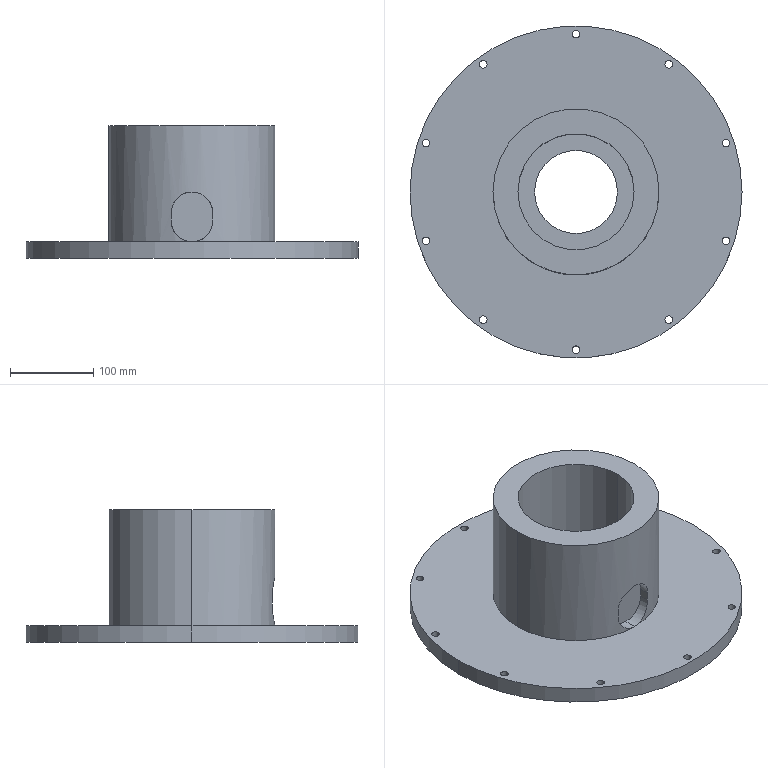Part | SolidWorks | features ICE 2, Cut 1, Extrusion 1, Fillet 1 | 1 solid | 39 faces | box 400 x 400 x 160 mm | volume 4551688 mm3 | cylinder 32 | plane 7 | commonest cylinder face diameters 9 x20 50 x4 100 x2 140 x2 200 x2 400 x2
STEP:
#1=CARTESIAN_POINT('',(-50.,0.,0.));
#2=VERTEX_POINT('',#1);
#3=CARTESIAN_POINT('',(50.,0.,0.));
#4=VERTEX_POINT('',#3);
#5=CARTESIAN_POINT('',(0.,0.,0.));
#6=DIRECTION('',(0.,0.,1.));
#7=DIRECTION('',(1.,0.,0.));
#8=AXIS2_PLACEMENT_3D('',#5,#6,#7);
#9=CIRCLE('',#8,50.);
#10=EDGE_CURVE('',#2,#4,#9,.T.);
#11=ORIENTED_EDGE('',*,*,#10,.F.);
#12=CARTESIAN_POINT('',(-50.,0.,20.));
#13=VERTEX_POINT('',#12);
#14=CARTESIAN_POINT('',(-50.,0.,0.));
#15=DIRECTION('',(0.,0.,1.));
#16=VECTOR('',#15,1000.);
#17=LINE('',#14,#16);
#18=EDGE_CURVE('',#2,#13,#17,.T.);
#19=ORIENTED_EDGE('',*,*,#18,.T.);
#20=CARTESIAN_POINT('',(50.,0.,20.));
#21=VERTEX_POINT('',#20);
#22=CARTESIAN_POINT('',(0.,0.,20.));
#23=DIRECTION('',(0.,0.,1.));
#24=DIRECTION('',(1.,0.,0.));
#25=AXIS2_PLACEMENT_3D('',#22,#23,#24);
#26=CIRCLE('',#25,50.);
#27=EDGE_CURVE('',#13,#21,#26,.T.);
#28=ORIENTED_EDGE('',*,*,#27,.T.);
#29=CARTESIAN_POINT('',(50.,0.,0.));
#30=DIRECTION('',(0.,0.,1.));
#31=VECTOR('',#30,1000.);
#32=LINE('',#29,#31);
#33=EDGE_CURVE('',#4,#21,#32,.T.);
#34=ORIENTED_EDGE('',*,*,#33,.F.);
#35=EDGE_LOOP('',(#11,#19,#28,#34));
#36=FACE_OUTER_BOUND('',#35,.T.);
#37=CARTESIAN_POINT('',(0.,0.,0.));
#38=DIRECTION('',(0.,0.,1.));
#39=DIRECTION('',(1.,0.,0.));
#40=AXIS2_PLACEMENT_3D('',#37,#38,#39);
#41=CYLINDRICAL_SURFACE('',#40,50.);
#42=ADVANCED_FACE('',(#36),#41,.F.);
#43=CARTESIAN_POINT('',(-70.,0.,160.));
#44=VERTEX_POINT('',#43);
#45=CARTESIAN_POINT('',(70.,0.,160.));
#46=VERTEX_POINT('',#45);
#47=CARTESIAN_POINT('',(0.,0.,160.));
#48=DIRECTION('',(0.,0.,1.));
#49=DIRECTION('',(1.,0.,0.));
#50=AXIS2_PLACEMENT_3D('',#47,#48,#49);
#51=CIRCLE('',#50,70.);
#52=EDGE_CURVE('',#44,#46,#51,.T.);
#53=ORIENTED_EDGE('',*,*,#52,.T.);
#54=CARTESIAN_POINT('',(70.,0.,20.));
#55=VERTEX_POINT('',#54);
#56=CARTESIAN_POINT('',(70.,0.,160.));
#57=DIRECTION('',(0.,0.,-1.));
#58=VECTOR('',#57,1000.);
#59=LINE('',#56,#58);
#60=EDGE_CURVE('',#46,#55,#59,.T.);
#61=ORIENTED_EDGE('',*,*,#60,.T.);
#62=CARTESIAN_POINT('',(-70.,0.,20.));
#63=VERTEX_POINT('',#62);
#64=CARTESIAN_POINT('',(0.,0.,20.));
#65=DIRECTION('',(0.,0.,-1.));
#66=DIRECTION('',(1.,0.,0.));
#67=AXIS2_PLACEMENT_3D('',#64,#65,#66);
#68=CIRCLE('',#67,70.);
#69=EDGE_CURVE('',#55,#63,#68,.T.);
#70=ORIENTED_EDGE('',*,*,#69,.T.);
#71=CARTESIAN_POINT('',(-70.,0.,160.));
#72=DIRECTION('',(0.,0.,-1.));
#73=VECTOR('',#72,1000.);
#74=LINE('',#71,#73);
#75=EDGE_CURVE('',#44,#63,#74,.T.);
#76=ORIENTED_EDGE('',*,*,#75,.F.);
#77=EDGE_LOOP('',(#53,#61,#70,#76));
#78=FACE_OUTER_BOUND('',#77,.T.);
#79=CARTESIAN_POINT('',(0.,0.,160.));
#80=DIRECTION('',(0.,0.,-1.));
#81=DIRECTION('',(-1.,0.,0.));
#82=AXIS2_PLACEMENT_3D('',#79,#80,#81);
#83=CYLINDRICAL_SURFACE('',#82,70.);
#84=ADVANCED_FACE('',(#78),#83,.F.);
#85=CARTESIAN_POINT('',(100.,0.,160.));
#86=VERTEX_POINT('',#85);
#87=CARTESIAN_POINT('',(-100.,0.,160.));
#88=VERTEX_POINT('',#87);
#89=CARTESIAN_POINT('',(0.,0.,160.));
#90=DIRECTION('',(0.,0.,1.));
#91=DIRECTION('',(1.,0.,0.));
#92=AXIS2_PLACEMENT_3D('',#89,#90,#91);
#93=CIRCLE('',#92,100.);
#94=EDGE_CURVE('',#86,#88,#93,.T.);
#95=ORIENTED_EDGE('',*,*,#94,.F.);
#96=CARTESIAN_POINT('',(100.,0.,20.));
#97=VERTEX_POINT('',#96);
#98=CARTESIAN_POINT('',(100.,0.,160.));
#99=DIRECTION('',(0.,0.,-1.));
#100=VECTOR('',#99,1000.);
#101=LINE('',#98,#100);
#102=EDGE_CURVE('',#86,#97,#101,.T.);
#103=ORIENTED_EDGE('',*,*,#102,.T.);
#104=CARTESIAN_POINT('',(-100.,0.,20.));
#105=VERTEX_POINT('',#104);
#106=CARTESIAN_POINT('',(0.,0.,20.));
#107=DIRECTION('',(0.,0.,1.));
#108=DIRECTION('',(1.,0.,0.));
#109=AXIS2_PLACEMENT_3D('',#106,#107,#108);
#110=CIRCLE('',#109,100.);
#111=EDGE_CURVE('',#97,#105,#110,.T.);
#112=ORIENTED_EDGE('',*,*,#111,.T.);
#113=CARTESIAN_POINT('',(-100.,0.,160.));
#114=DIRECTION('',(0.,0.,-1.));
#115=VECTOR('',#114,1000.);
#116=LINE('',#113,#115);
#117=EDGE_CURVE('',#88,#105,#116,.T.);
#118=ORIENTED_EDGE('',*,*,#117,.F.);
#119=EDGE_LOOP('',(#95,#103,#112,#118));
#120=FACE_OUTER_BOUND('',#119,.T.);
#121=CARTESIAN_POINT('',(0.,0.,160.));
#122=DIRECTION('',(0.,0.,-1.));
#123=DIRECTION('',(-1.,0.,0.));
#124=AXIS2_PLACEMENT_3D('',#121,#122,#123);
#125=CYLINDRICAL_SURFACE('',#124,100.);
#126=ADVANCED_FACE('',(#120),#125,.T.);
#127=CARTESIAN_POINT('',(-116.179,153.713,20.));
#128=VERTEX_POINT('',#127);
#129=CARTESIAN_POINT('',(-107.179,153.713,20.));
#130=VERTEX_POINT('',#129);
#131=CARTESIAN_POINT('',(-111.679,153.713,20.));
#132=DIRECTION('',(0.,0.,1.));
#133=DIRECTION('',(1.,0.,0.));
#134=AXIS2_PLACEMENT_3D('',#131,#132,#133);
#135=CIRCLE('',#134,4.5);
#136=EDGE_CURVE('',#128,#130,#135,.T.);
#137=ORIENTED_EDGE('',*,*,#136,.T.);
#138=CARTESIAN_POINT('',(-107.179,153.713,0.));
#139=VERTEX_POINT('',#138);
#140=CARTESIAN_POINT('',(-107.179,153.713,20.));
#141=DIRECTION('',(0.,0.,-1.));
#142=VECTOR('',#141,1000.);
#143=LINE('',#140,#142);
#144=EDGE_CURVE('',#130,#139,#143,.T.);
#145=ORIENTED_EDGE('',*,*,#144,.T.);
#146=CARTESIAN_POINT('',(-116.179,153.713,0.));
#147=VERTEX_POINT('',#146);
#148=CARTESIAN_POINT('',(-111.679,153.713,0.));
#149=DIRECTION('',(0.,0.,1.));
#150=DIRECTION('',(1.,0.,0.));
#151=AXIS2_PLACEMENT_3D('',#148,#149,#150);
#152=CIRCLE('',#151,4.5);
#153=EDGE_CURVE('',#147,#139,#152,.T.);
#154=ORIENTED_EDGE('',*,*,#153,.F.);
#155=CARTESIAN_POINT('',(-116.179,153.713,20.));
#156=DIRECTION('',(0.,0.,-1.));
#157=VECTOR('',#156,1000.);
#158=LINE('',#155,#157);
#159=EDGE_CURVE('',#128,#147,#158,.T.);
#160=ORIENTED_EDGE('',*,*,#159,.F.);
#161=EDGE_LOOP('',(#137,#145,#154,#160));
#162=FACE_OUTER_BOUND('',#161,.T.);
#163=CARTESIAN_POINT('',(-111.679,153.713,20.));
#164=DIRECTION('',(0.,0.,-1.));
#165=DIRECTION('',(-1.,0.,0.));
#166=AXIS2_PLACEMENT_3D('',#163,#164,#165);
#167=CYLINDRICAL_SURFACE('',#166,4.5);
#168=ADVANCED_FACE('',(#162),#167,.F.);
#169=CARTESIAN_POINT('',(-185.201,58.713,20.));
#170=VERTEX_POINT('',#169);
#171=CARTESIAN_POINT('',(-176.201,58.713,20.));
#172=VERTEX_POINT('',#171);
#173=CARTESIAN_POINT('',(-180.701,58.713,20.));
#174=DIRECTION('',(0.,0.,1.));
#175=DIRECTION('',(1.,0.,0.));
#176=AXIS2_PLACEMENT_3D('',#173,#174,#175);
#177=CIRCLE('',#176,4.5);
#178=EDGE_CURVE('',#170,#172,#177,.T.);
#179=ORIENTED_EDGE('',*,*,#178,.T.);
#180=CARTESIAN_POINT('',(-176.201,58.713,0.));
#181=VERTEX_POINT('',#180);
#182=CARTESIAN_POINT('',(-176.201,58.713,20.));
#183=DIRECTION('',(0.,0.,-1.));
#184=VECTOR('',#183,1000.);
#185=LINE('',#182,#184);
#186=EDGE_CURVE('',#172,#181,#185,.T.);
#187=ORIENTED_EDGE('',*,*,#186,.T.);
#188=CARTESIAN_POINT('',(-185.201,58.713,0.));
#189=VERTEX_POINT('',#188);
#190=CARTESIAN_POINT('',(-180.701,58.713,0.));
#191=DIRECTION('',(0.,0.,1.));
#192=DIRECTION('',(1.,0.,0.));
#193=AXIS2_PLACEMENT_3D('',#190,#191,#192);
#194=CIRCLE('',#193,4.5);
#195=EDGE_CURVE('',#189,#181,#194,.T.);
#196=ORIENTED_EDGE('',*,*,#195,.F.);
#197=CARTESIAN_POINT('',(-185.201,58.713,20.));
#198=DIRECTION('',(0.,0.,-1.));
#199=VECTOR('',#198,1000.);
#200=LINE('',#197,#199);
#201=EDGE_CURVE('',#170,#189,#200,.T.);
#202=ORIENTED_EDGE('',*,*,#201,.F.);
#203=EDGE_LOOP('',(#179,#187,#196,#202));
#204=FACE_OUTER_BOUND('',#203,.T.);
#205=CARTESIAN_POINT('',(-180.701,58.713,20.));
#206=DIRECTION('',(0.,0.,-1.));
#207=DIRECTION('',(-1.,0.,0.));
#208=AXIS2_PLACEMENT_3D('',#205,#206,#207);
#209=CYLINDRICAL_SURFACE('',#208,4.5);
#210=ADVANCED_FACE('',(#204),#209,.F.);
#211=CARTESIAN_POINT('',(-185.201,-58.713,20.));
#212=VERTEX_POINT('',#211);
#213=CARTESIAN_POINT('',(-176.201,-58.713,20.));
#214=VERTEX_POINT('',#213);
#215=CARTESIAN_POINT('',(-180.701,-58.713,20.));
#216=DIRECTION('',(0.,0.,1.));
#217=DIRECTION('',(1.,0.,0.));
#218=AXIS2_PLACEMENT_3D('',#215,#216,#217);
#219=CIRCLE('',#218,4.5);
#220=EDGE_CURVE('',#212,#214,#219,.T.);
#221=ORIENTED_EDGE('',*,*,#220,.T.);
#222=CARTESIAN_POINT('',(-176.201,-58.713,0.));
#223=VERTEX_POINT('',#222);
#224=CARTESIAN_POINT('',(-176.201,-58.713,20.));
#225=DIRECTION('',(0.,0.,-1.));
#226=VECTOR('',#225,1000.);
#227=LINE('',#224,#226);
#228=EDGE_CURVE('',#214,#223,#227,.T.);
#229=ORIENTED_EDGE('',*,*,#228,.T.);
#230=CARTESIAN_POINT('',(-185.201,-58.713,0.));
#231=VERTEX_POINT('',#230);
#232=CARTESIAN_POINT('',(-180.701,-58.713,0.));
#233=DIRECTION('',(0.,0.,1.));
#234=DIRECTION('',(1.,0.,0.));
#235=AXIS2_PLACEMENT_3D('',#232,#233,#234);
#236=CIRCLE('',#235,4.5);
#237=EDGE_CURVE('',#231,#223,#236,.T.);
#238=ORIENTED_EDGE('',*,*,#237,.F.);
#239=CARTESIAN_POINT('',(-185.201,-58.713,20.));
#240=DIRECTION('',(0.,0.,-1.));
#241=VECTOR('',#240,1000.);
#242=LINE('',#239,#241);
#243=EDGE_CURVE('',#212,#231,#242,.T.);
#244=ORIENTED_EDGE('',*,*,#243,.F.);
#245=EDGE_LOOP('',(#221,#229,#238,#244));
#246=FACE_OUTER_BOUND('',#245,.T.);
#247=CARTESIAN_POINT('',(-180.701,-58.713,20.));
#248=DIRECTION('',(0.,0.,-1.));
#249=DIRECTION('',(-1.,0.,0.));
#250=AXIS2_PLACEMENT_3D('',#247,#248,#249);
#251=CYLINDRICAL_SURFACE('',#250,4.5);
#252=ADVANCED_FACE('',(#246),#251,.F.);
#253=CARTESIAN_POINT('',(-116.179,-153.713,20.));
#254=VERTEX_POINT('',#253);
#255=CARTESIAN_POINT('',(-107.179,-153.713,20.));
#256=VERTEX_POINT('',#255);
#257=CARTESIAN_POINT('',(-111.679,-153.713,20.));
#258=DIRECTION('',(0.,0.,1.));
#259=DIRECTION('',(1.,0.,0.));
#260=AXIS2_PLACEMENT_3D('',#257,#258,#259);
#261=CIRCLE('',#260,4.5);
#262=EDGE_CURVE('',#254,#256,#261,.T.);
#263=ORIENTED_EDGE('',*,*,#262,.T.);
#264=CARTESIAN_POINT('',(-107.179,-153.713,0.));
#265=VERTEX_POINT('',#264);
#266=CARTESIAN_POINT('',(-107.179,-153.713,20.));
#267=DIRECTION('',(0.,0.,-1.));
#268=VECTOR('',#267,1000.);
#269=LINE('',#266,#268);
#270=EDGE_CURVE('',#256,#265,#269,.T.);
#271=ORIENTED_EDGE('',*,*,#270,.T.);
#272=CARTESIAN_POINT('',(-116.179,-153.713,0.));
#273=VERTEX_POINT('',#272);
#274=CARTESIAN_POINT('',(-111.679,-153.713,0.));
#275=DIRECTION('',(0.,0.,1.));
#276=DIRECTION('',(1.,0.,0.));
#277=AXIS2_PLACEMENT_3D('',#274,#275,#276);
#278=CIRCLE('',#277,4.5);
#279=EDGE_CURVE('',#273,#265,#278,.T.);
#280=ORIENTED_EDGE('',*,*,#279,.F.);
#281=CARTESIAN_POINT('',(-116.179,-153.713,20.));
#282=DIRECTION('',(0.,0.,-1.));
#283=VECTOR('',#282,1000.);
#284=LINE('',#281,#283);
#285=EDGE_CURVE('',#254,#273,#284,.T.);
#286=ORIENTED_EDGE('',*,*,#285,.F.);
#287=EDGE_LOOP('',(#263,#271,#280,#286));
#288=FACE_OUTER_BOUND('',#287,.T.);
#289=CARTESIAN_POINT('',(-111.679,-153.713,20.));
#290=DIRECTION('',(0.,0.,-1.));
#291=DIRECTION('',(-1.,0.,0.));
#292=AXIS2_PLACEMENT_3D('',#289,#290,#291);
#293=CYLINDRICAL_SURFACE('',#292,4.5);
#294=ADVANCED_FACE('',(#288),#293,.F.);
#295=CARTESIAN_POINT('',(-4.5,-190.,20.));
#296=VERTEX_POINT('',#295);
#297=CARTESIAN_POINT('',(4.5,-190.,20.));
#298=VERTEX_POINT('',#297);
#299=CARTESIAN_POINT('',(0.,-190.,20.));
#300=DIRECTION('',(0.,0.,1.));
#301=DIRECTION('',(1.,0.,0.));
#302=AXIS2_PLACEMENT_3D('',#299,#300,#301);
#303=CIRCLE('',#302,4.5);
#304=EDGE_CURVE('',#296,#298,#303,.T.);
#305=ORIENTED_EDGE('',*,*,#304,.T.);
#306=CARTESIAN_POINT('',(4.5,-190.,0.));
#307=VERTEX_POINT('',#306);
#308=CARTESIAN_POINT('',(4.5,-190.,20.));
#309=DIRECTION('',(0.,0.,-1.));
#310=VECTOR('',#309,1000.);
#311=LINE('',#308,#310);
#312=EDGE_CURVE('',#298,#307,#311,.T.);
#313=ORIENTED_EDGE('',*,*,#312,.T.);
#314=CARTESIAN_POINT('',(-4.5,-190.,0.));
#315=VERTEX_POINT('',#314);
#316=CARTESIAN_POINT('',(0.,-190.,0.));
#317=DIRECTION('',(0.,0.,1.));
#318=DIRECTION('',(1.,0.,0.));
#319=AXIS2_PLACEMENT_3D('',#316,#317,#318);
#320=CIRCLE('',#319,4.5);
#321=EDGE_CURVE('',#315,#307,#320,.T.);
#322=ORIENTED_EDGE('',*,*,#321,.F.);
#323=CARTESIAN_POINT('',(-4.5,-190.,20.));
#324=DIRECTION('',(0.,0.,-1.));
#325=VECTOR('',#324,1000.);
#326=LINE('',#323,#325);
#327=EDGE_CURVE('',#296,#315,#326,.T.);
#328=ORIENTED_EDGE('',*,*,#327,.F.);
#329=EDGE_LOOP('',(#305,#313,#322,#328));
#330=FACE_OUTER_BOUND('',#329,.T.);
#331=CARTESIAN_POINT('',(0.,-190.,20.));
#332=DIRECTION('',(0.,0.,-1.));
#333=DIRECTION('',(-1.,0.,0.));
#334=AXIS2_PLACEMENT_3D('',#331,#332,#333);
#335=CYLINDRICAL_SURFACE('',#334,4.5);
#336=ADVANCED_FACE('',(#330),#335,.F.);
#337=CARTESIAN_POINT('',(107.179,-153.713,20.));
#338=VERTEX_POINT('',#337);
#339=CARTESIAN_POINT('',(116.179,-153.713,20.));
#340=VERTEX_POINT('',#339);
#341=CARTESIAN_POINT('',(111.679,-153.713,20.));
#342=DIRECTION('',(0.,0.,1.));
#343=DIRECTION('',(1.,0.,0.));
#344=AXIS2_PLACEMENT_3D('',#341,#342,#343);
#345=CIRCLE('',#344,4.5);
#346=EDGE_CURVE('',#338,#340,#345,.T.);
#347=ORIENTED_EDGE('',*,*,#346,.T.);
#348=CARTESIAN_POINT('',(116.179,-153.713,0.));
#349=VERTEX_POINT('',#348);
#350=CARTESIAN_POINT('',(116.179,-153.713,20.));
#351=DIRECTION('',(0.,0.,-1.));
#352=VECTOR('',#351,1000.);
#353=LINE('',#350,#352);
#354=EDGE_CURVE('',#340,#349,#353,.T.);
#355=ORIENTED_EDGE('',*,*,#354,.T.);
#356=CARTESIAN_POINT('',(107.179,-153.713,0.));
#357=VERTEX_POINT('',#356);
#358=CARTESIAN_POINT('',(111.679,-153.713,0.));
#359=DIRECTION('',(0.,0.,1.));
#360=DIRECTION('',(1.,0.,0.));
#361=AXIS2_PLACEMENT_3D('',#358,#359,#360);
#362=CIRCLE('',#361,4.5);
#363=EDGE_CURVE('',#357,#349,#362,.T.);
#364=ORIENTED_EDGE('',*,*,#363,.F.);
#365=CARTESIAN_POINT('',(107.179,-153.713,20.));
#366=DIRECTION('',(0.,0.,-1.));
#367=VECTOR('',#366,1000.);
#368=LINE('',#365,#367);
#369=EDGE_CURVE('',#338,#357,#368,.T.);
#370=ORIENTED_EDGE('',*,*,#369,.F.);
#371=EDGE_LOOP('',(#347,#355,#364,#370));
#372=FACE_OUTER_BOUND('',#371,.T.);
#373=CARTESIAN_POINT('',(111.679,-153.713,20.));
#374=DIRECTION('',(0.,0.,-1.));
#375=DIRECTION('',(-1.,0.,0.));
#376=AXIS2_PLACEMENT_3D('',#373,#374,#375);
#377=CYLINDRICAL_SURFACE('',#376,4.5);
#378=ADVANCED_FACE('',(#372),#377,.F.);
#379=CARTESIAN_POINT('',(176.201,-58.713,20.));
#380=VERTEX_POINT('',#379);
#381=CARTESIAN_POINT('',(185.201,-58.713,20.));
#382=VERTEX_POINT('',#381);
#383=CARTESIAN_POINT('',(180.701,-58.713,20.));
#384=DIRECTION('',(0.,0.,1.));
#385=DIRECTION('',(1.,0.,0.));
#386=AXIS2_PLACEMENT_3D('',#383,#384,#385);
#387=CIRCLE('',#386,4.5);
#388=EDGE_CURVE('',#380,#382,#387,.T.);
#389=ORIENTED_EDGE('',*,*,#388,.T.);
#390=CARTESIAN_POINT('',(185.201,-58.713,0.));
#391=VERTEX_POINT('',#390);
#392=CARTESIAN_POINT('',(185.201,-58.713,20.));
#393=DIRECTION('',(0.,0.,-1.));
#394=VECTOR('',#393,1000.);
#395=LINE('',#392,#394);
#396=EDGE_CURVE('',#382,#391,#395,.T.);
#397=ORIENTED_EDGE('',*,*,#396,.T.);
#398=CARTESIAN_POINT('',(176.201,-58.713,0.));
#399=VERTEX_POINT('',#398);
#400=CARTESIAN_POINT('',(180.701,-58.713,0.));
#401=DIRECTION('',(0.,0.,1.));
#402=DIRECTION('',(1.,0.,0.));
#403=AXIS2_PLACEMENT_3D('',#400,#401,#402);
#404=CIRCLE('',#403,4.5);
#405=EDGE_CURVE('',#399,#391,#404,.T.);
#406=ORIENTED_EDGE('',*,*,#405,.F.);
#407=CARTESIAN_POINT('',(176.201,-58.713,20.));
#408=DIRECTION('',(0.,0.,-1.));
#409=VECTOR('',#408,1000.);
#410=LINE('',#407,#409);
#411=EDGE_CURVE('',#380,#399,#410,.T.);
#412=ORIENTED_EDGE('',*,*,#411,.F.);
#413=EDGE_LOOP('',(#389,#397,#406,#412));
#414=FACE_OUTER_BOUND('',#413,.T.);
#415=CARTESIAN_POINT('',(180.701,-58.713,20.));
#416=DIRECTION('',(0.,0.,-1.));
#417=DIRECTION('',(-1.,0.,0.));
#418=AXIS2_PLACEMENT_3D('',#415,#416,#417);
#419=CYLINDRICAL_SURFACE('',#418,4.5);
#420=ADVANCED_FACE('',(#414),#419,.F.);
#421=CARTESIAN_POINT('',(176.201,58.713,20.));
#422=VERTEX_POINT('',#421);
#423=CARTESIAN_POINT('',(185.201,58.713,20.));
#424=VERTEX_POINT('',#423);
#425=CARTESIAN_POINT('',(180.701,58.713,20.));
#426=DIRECTION('',(0.,0.,1.));
#427=DIRECTION('',(1.,0.,0.));
#428=AXIS2_PLACEMENT_3D('',#425,#426,#427);
#429=CIRCLE('',#428,4.5);
#430=EDGE_CURVE('',#422,#424,#429,.T.);
#431=ORIENTED_EDGE('',*,*,#430,.T.);
#432=CARTESIAN_POINT('',(185.201,58.713,0.));
#433=VERTEX_POINT('',#432);
#434=CARTESIAN_POINT('',(185.201,58.713,20.));
#435=DIRECTION('',(0.,0.,-1.));
#436=VECTOR('',#435,1000.);
#437=LINE('',#434,#436);
#438=EDGE_CURVE('',#424,#433,#437,.T.);
#439=ORIENTED_EDGE('',*,*,#438,.T.);
#440=CARTESIAN_POINT('',(176.201,58.713,0.));
#441=VERTEX_POINT('',#440);
#442=CARTESIAN_POINT('',(180.701,58.713,0.));
#443=DIRECTION('',(0.,0.,1.));
#444=DIRECTION('',(1.,0.,0.));
#445=AXIS2_PLACEMENT_3D('',#442,#443,#444);
#446=CIRCLE('',#445,4.5);
#447=EDGE_CURVE('',#441,#433,#446,.T.);
#448=ORIENTED_EDGE('',*,*,#447,.F.);
#449=CARTESIAN_POINT('',(176.201,58.713,20.));
#450=DIRECTION('',(0.,0.,-1.));
#451=VECTOR('',#450,1000.);
#452=LINE('',#449,#451);
#453=EDGE_CURVE('',#422,#441,#452,.T.);
#454=ORIENTED_EDGE('',*,*,#453,.F.);
#455=EDGE_LOOP('',(#431,#439,#448,#454));
#456=FACE_OUTER_BOUND('',#455,.T.);
#457=CARTESIAN_POINT('',(180.701,58.713,20.));
#458=DIRECTION('',(0.,0.,-1.));
#459=DIRECTION('',(-1.,0.,0.));
#460=AXIS2_PLACEMENT_3D('',#457,#458,#459);
#461=CYLINDRICAL_SURFACE('',#460,4.5);
#462=ADVANCED_FACE('',(#456),#461,.F.);
#463=CARTESIAN_POINT('',(107.179,153.713,20.));
#464=VERTEX_POINT('',#463);
#465=CARTESIAN_POINT('',(116.179,153.713,20.));
#466=VERTEX_POINT('',#465);
#467=CARTESIAN_POINT('',(111.679,153.713,20.));
#468=DIRECTION('',(0.,0.,1.));
#469=DIRECTION('',(1.,0.,0.));
#470=AXIS2_PLACEMENT_3D('',#467,#468,#469);
#471=CIRCLE('',#470,4.5);
#472=EDGE_CURVE('',#464,#466,#471,.T.);
#473=ORIENTED_EDGE('',*,*,#472,.T.);
#474=CARTESIAN_POINT('',(116.179,153.713,0.));
#475=VERTEX_POINT('',#474);
#476=CARTESIAN_POINT('',(116.179,153.713,20.));
#477=DIRECTION('',(0.,0.,-1.));
#478=VECTOR('',#477,1000.);
#479=LINE('',#476,#478);
#480=EDGE_CURVE('',#466,#475,#479,.T.);
#481=ORIENTED_EDGE('',*,*,#480,.T.);
#482=CARTESIAN_POINT('',(107.179,153.713,0.));
#483=VERTEX_POINT('',#482);
#484=CARTESIAN_POINT('',(111.679,153.713,0.));
#485=DIRECTION('',(0.,0.,1.));
#486=DIRECTION('',(1.,0.,0.));
#487=AXIS2_PLACEMENT_3D('',#484,#485,#486);
#488=CIRCLE('',#487,4.5);
#489=EDGE_CURVE('',#483,#475,#488,.T.);
#490=ORIENTED_EDGE('',*,*,#489,.F.);
#491=CARTESIAN_POINT('',(107.179,153.713,20.));
#492=DIRECTION('',(0.,0.,-1.));
#493=VECTOR('',#492,1000.);
#494=LINE('',#491,#493);
#495=EDGE_CURVE('',#464,#483,#494,.T.);
#496=ORIENTED_EDGE('',*,*,#495,.F.);
#497=EDGE_LOOP('',(#473,#481,#490,#496));
#498=FACE_OUTER_BOUND('',#497,.T.);
#499=CARTESIAN_POINT('',(111.679,153.713,20.));
#500=DIRECTION('',(0.,0.,-1.));
#501=DIRECTION('',(-1.,0.,0.));
#502=AXIS2_PLACEMENT_3D('',#499,#500,#501);
#503=CYLINDRICAL_SURFACE('',#502,4.5);
#504=ADVANCED_FACE('',(#498),#503,.F.);
#505=CARTESIAN_POINT('',(-4.5,190.,20.));
#506=VERTEX_POINT('',#505);
#507=CARTESIAN_POINT('',(4.5,190.,20.));
#508=VERTEX_POINT('',#507);
#509=CARTESIAN_POINT('',(0.,190.,20.));
#510=DIRECTION('',(0.,0.,1.));
#511=DIRECTION('',(1.,0.,0.));
#512=AXIS2_PLACEMENT_3D('',#509,#510,#511);
#513=CIRCLE('',#512,4.5);
#514=EDGE_CURVE('',#506,#508,#513,.T.);
#515=ORIENTED_EDGE('',*,*,#514,.T.);
#516=CARTESIAN_POINT('',(4.5,190.,0.));
#517=VERTEX_POINT('',#516);
#518=CARTESIAN_POINT('',(4.5,190.,20.));
#519=DIRECTION('',(0.,0.,-1.));
#520=VECTOR('',#519,1000.);
#521=LINE('',#518,#520);
#522=EDGE_CURVE('',#508,#517,#521,.T.);
#523=ORIENTED_EDGE('',*,*,#522,.T.);
#524=CARTESIAN_POINT('',(-4.5,190.,0.));
#525=VERTEX_POINT('',#524);
#526=CARTESIAN_POINT('',(0.,190.,0.));
#527=DIRECTION('',(0.,0.,1.));
#528=DIRECTION('',(1.,0.,0.));
#529=AXIS2_PLACEMENT_3D('',#526,#527,#528);
#530=CIRCLE('',#529,4.5);
#531=EDGE_CURVE('',#525,#517,#530,.T.);
#532=ORIENTED_EDGE('',*,*,#531,.F.);
#533=CARTESIAN_POINT('',(-4.5,190.,20.));
#534=DIRECTION('',(0.,0.,-1.));
#535=VECTOR('',#534,1000.);
#536=LINE('',#533,#535);
#537=EDGE_CURVE('',#506,#525,#536,.T.);
#538=ORIENTED_EDGE('',*,*,#537,.F.);
#539=EDGE_LOOP('',(#515,#523,#532,#538));
#540=FACE_OUTER_BOUND('',#539,.T.);
#541=CARTESIAN_POINT('',(0.,190.,20.));
#542=DIRECTION('',(0.,0.,-1.));
#543=DIRECTION('',(-1.,0.,0.));
#544=AXIS2_PLACEMENT_3D('',#541,#542,#543);
#545=CYLINDRICAL_SURFACE('',#544,4.5);
#546=ADVANCED_FACE('',(#540),#545,.F.);
#547=CARTESIAN_POINT('',(200.,0.,20.));
#548=VERTEX_POINT('',#547);
#549=CARTESIAN_POINT('',(-200.,0.,20.));
#550=VERTEX_POINT('',#549);
#551=CARTESIAN_POINT('',(0.,0.,20.));
#552=DIRECTION('',(0.,0.,1.));
#553=DIRECTION('',(1.,0.,0.));
#554=AXIS2_PLACEMENT_3D('',#551,#552,#553);
#555=CIRCLE('',#554,200.);
#556=EDGE_CURVE('',#548,#550,#555,.T.);
#557=ORIENTED_EDGE('',*,*,#556,.F.);
#558=CARTESIAN_POINT('',(200.,0.,0.));
#559=VERTEX_POINT('',#558);
#560=CARTESIAN_POINT('',(200.,0.,20.));
#561=DIRECTION('',(0.,0.,-1.));
#562=VECTOR('',#561,1000.);
#563=LINE('',#560,#562);
#564=EDGE_CURVE('',#548,#559,#563,.T.);
#565=ORIENTED_EDGE('',*,*,#564,.T.);
#566=CARTESIAN_POINT('',(-200.,0.,0.));
#567=VERTEX_POINT('',#566);
#568=CARTESIAN_POINT('',(0.,0.,0.));
#569=DIRECTION('',(0.,0.,1.));
#570=DIRECTION('',(1.,0.,0.));
#571=AXIS2_PLACEMENT_3D('',#568,#569,#570);
#572=CIRCLE('',#571,200.);
#573=EDGE_CURVE('',#559,#567,#572,.T.);
#574=ORIENTED_EDGE('',*,*,#573,.T.);
#575=CARTESIAN_POINT('',(-200.,0.,20.));
#576=DIRECTION('',(0.,0.,-1.));
#577=VECTOR('',#576,1000.);
#578=LINE('',#575,#577);
#579=EDGE_CURVE('',#550,#567,#578,.T.);
#580=ORIENTED_EDGE('',*,*,#579,.F.);
#581=EDGE_LOOP('',(#557,#565,#574,#580));
#582=FACE_OUTER_BOUND('',#581,.T.);
#583=CARTESIAN_POINT('',(0.,0.,20.));
#584=DIRECTION('',(0.,0.,-1.));
#585=DIRECTION('',(-1.,0.,0.));
#586=AXIS2_PLACEMENT_3D('',#583,#584,#585);
#587=CYLINDRICAL_SURFACE('',#586,200.);
#588=ADVANCED_FACE('',(#582),#587,.T.);
#589=CARTESIAN_POINT('',(0.,0.,20.));
#590=DIRECTION('',(0.,0.,1.));
#591=DIRECTION('',(1.,0.,0.));
#592=AXIS2_PLACEMENT_3D('',#589,#590,#591);
#593=CIRCLE('',#592,200.);
#594=EDGE_CURVE('',#550,#548,#593,.T.);
#595=ORIENTED_EDGE('',*,*,#594,.T.);
#596=ORIENTED_EDGE('',*,*,#556,.T.);
#597=EDGE_LOOP('',(#595,#596));
#598=FACE_OUTER_BOUND('',#597,.T.);
#599=CARTESIAN_POINT('',(0.,-100.,20.));
#600=VERTEX_POINT('',#599);
#601=CARTESIAN_POINT('',(0.,0.,20.));
#602=DIRECTION('',(0.,0.,1.));
#603=DIRECTION('',(1.,0.,0.));
#604=AXIS2_PLACEMENT_3D('',#601,#602,#603);
#605=CIRCLE('',#604,100.);
#606=EDGE_CURVE('',#600,#97,#605,.T.);
#607=ORIENTED_EDGE('',*,*,#606,.F.);
#608=CARTESIAN_POINT('',(0.,0.,20.));
#609=DIRECTION('',(0.,0.,1.));
#610=DIRECTION('',(1.,0.,0.));
#611=AXIS2_PLACEMENT_3D('',#608,#609,#610);
#612=CIRCLE('',#611,100.);
#613=EDGE_CURVE('',#105,#600,#612,.T.);
#614=ORIENTED_EDGE('',*,*,#613,.F.);
#615=ORIENTED_EDGE('',*,*,#111,.F.);
#616=EDGE_LOOP('',(#607,#614,#615));
#617=FACE_BOUND('',#616,.T.);
#618=ORIENTED_EDGE('',*,*,#178,.F.);
#619=CARTESIAN_POINT('',(-180.701,58.713,20.));
#620=DIRECTION('',(0.,0.,1.));
#621=DIRECTION('',(1.,0.,0.));
#622=AXIS2_PLACEMENT_3D('',#619,#620,#621);
#623=CIRCLE('',#622,4.5);
#624=EDGE_CURVE('',#172,#170,#623,.T.);
#625=ORIENTED_EDGE('',*,*,#624,.F.);
#626=EDGE_LOOP('',(#618,#625));
#627=FACE_BOUND('',#626,.T.);
#628=ORIENTED_EDGE('',*,*,#262,.F.);
#629=CARTESIAN_POINT('',(-111.679,-153.713,20.));
#630=DIRECTION('',(0.,0.,1.));
#631=DIRECTION('',(1.,0.,0.));
#632=AXIS2_PLACEMENT_3D('',#629,#630,#631);
#633=CIRCLE('',#632,4.5);
#634=EDGE_CURVE('',#256,#254,#633,.T.);
#635=ORIENTED_EDGE('',*,*,#634,.F.);
#636=EDGE_LOOP('',(#628,#635));
#637=FACE_BOUND('',#636,.T.);
#638=ORIENTED_EDGE('',*,*,#346,.F.);
#639=CARTESIAN_POINT('',(111.679,-153.713,20.));
#640=DIRECTION('',(0.,0.,1.));
#641=DIRECTION('',(1.,0.,0.));
#642=AXIS2_PLACEMENT_3D('',#639,#640,#641);
#643=CIRCLE('',#642,4.5);
#644=EDGE_CURVE('',#340,#338,#643,.T.);
#645=ORIENTED_EDGE('',*,*,#644,.F.);
#646=EDGE_LOOP('',(#638,#645));
#647=FACE_BOUND('',#646,.T.);
#648=ORIENTED_EDGE('',*,*,#430,.F.);
#649=CARTESIAN_POINT('',(180.701,58.713,20.));
#650=DIRECTION('',(0.,0.,1.));
#651=DIRECTION('',(1.,0.,0.));
#652=AXIS2_PLACEMENT_3D('',#649,#650,#651);
#653=CIRCLE('',#652,4.5);
#654=EDGE_CURVE('',#424,#422,#653,.T.);
#655=ORIENTED_EDGE('',*,*,#654,.F.);
#656=EDGE_LOOP('',(#648,#655));
#657=FACE_BOUND('',#656,.T.);
#658=ORIENTED_EDGE('',*,*,#514,.F.);
#659=CARTESIAN_POINT('',(0.,190.,20.));
#660=DIRECTION('',(0.,0.,1.));
#661=DIRECTION('',(1.,0.,0.));
#662=AXIS2_PLACEMENT_3D('',#659,#660,#661);
#663=CIRCLE('',#662,4.5);
#664=EDGE_CURVE('',#508,#506,#663,.T.);
#665=ORIENTED_EDGE('',*,*,#664,.F.);
#666=EDGE_LOOP('',(#658,#665));
#667=FACE_BOUND('',#666,.T.);
#668=ORIENTED_EDGE('',*,*,#472,.F.);
#669=CARTESIAN_POINT('',(111.679,153.713,20.));
#670=DIRECTION('',(0.,0.,1.));
#671=DIRECTION('',(1.,0.,0.));
#672=AXIS2_PLACEMENT_3D('',#669,#670,#671);
#673=CIRCLE('',#672,4.5);
#674=EDGE_CURVE('',#466,#464,#673,.T.);
#675=ORIENTED_EDGE('',*,*,#674,.F.);
#676=EDGE_LOOP('',(#668,#675));
#677=FACE_BOUND('',#676,.T.);
#678=ORIENTED_EDGE('',*,*,#388,.F.);
#679=CARTESIAN_POINT('',(180.701,-58.713,20.));
#680=DIRECTION('',(0.,0.,1.));
#681=DIRECTION('',(1.,0.,0.));
#682=AXIS2_PLACEMENT_3D('',#679,#680,#681);
#683=CIRCLE('',#682,4.5);
#684=EDGE_CURVE('',#382,#380,#683,.T.);
#685=ORIENTED_EDGE('',*,*,#684,.F.);
#686=EDGE_LOOP('',(#678,#685));
#687=FACE_BOUND('',#686,.T.);
#688=ORIENTED_EDGE('',*,*,#220,.F.);
#689=CARTESIAN_POINT('',(-180.701,-58.713,20.));
#690=DIRECTION('',(0.,0.,1.));
#691=DIRECTION('',(1.,0.,0.));
#692=AXIS2_PLACEMENT_3D('',#689,#690,#691);
#693=CIRCLE('',#692,4.5);
#694=EDGE_CURVE('',#214,#212,#693,.T.);
#695=ORIENTED_EDGE('',*,*,#694,.F.);
#696=EDGE_LOOP('',(#688,#695));
#697=FACE_BOUND('',#696,.T.);
#698=ORIENTED_EDGE('',*,*,#136,.F.);
#699=CARTESIAN_POINT('',(-111.679,153.713,20.));
#700=DIRECTION('',(0.,0.,1.));
#701=DIRECTION('',(1.,0.,0.));
#702=AXIS2_PLACEMENT_3D('',#699,#700,#701);
#703=CIRCLE('',#702,4.5);
#704=EDGE_CURVE('',#130,#128,#703,.T.);
#705=ORIENTED_EDGE('',*,*,#704,.F.);
#706=EDGE_LOOP('',(#698,#705));
#707=FACE_BOUND('',#706,.T.);
#708=ORIENTED_EDGE('',*,*,#304,.F.);
#709=CARTESIAN_POINT('',(0.,-190.,20.));
#710=DIRECTION('',(0.,0.,1.));
#711=DIRECTION('',(1.,0.,0.));
#712=AXIS2_PLACEMENT_3D('',#709,#710,#711);
#713=CIRCLE('',#712,4.5);
#714=EDGE_CURVE('',#298,#296,#713,.T.);
#715=ORIENTED_EDGE('',*,*,#714,.F.);
#716=EDGE_LOOP('',(#708,#715));
#717=FACE_BOUND('',#716,.T.);
#718=CARTESIAN_POINT('',(0.,0.,20.));
#719=DIRECTION('',(0.,0.,1.));
#720=DIRECTION('',(1.,0.,0.));
#721=AXIS2_PLACEMENT_3D('',#718,#719,#720);
#722=PLANE('',#721);
#723=ADVANCED_FACE('',(#598,#617,#627,#637,#647,#657,#667,#677,#687,#697,#707,#717),#722,.T.);
#724=CARTESIAN_POINT('',(0.,0.,0.));
#725=DIRECTION('',(0.,0.,1.));
#726=DIRECTION('',(1.,0.,0.));
#727=AXIS2_PLACEMENT_3D('',#724,#725,#726);
#728=CIRCLE('',#727,50.);
#729=EDGE_CURVE('',#4,#2,#728,.T.);
#730=ORIENTED_EDGE('',*,*,#729,.T.);
#731=ORIENTED_EDGE('',*,*,#10,.T.);
#732=EDGE_LOOP('',(#730,#731));
#733=FACE_BOUND('',#732,.T.);
#734=CARTESIAN_POINT('',(0.,0.,0.));
#735=DIRECTION('',(0.,0.,1.));
#736=DIRECTION('',(1.,0.,0.));
#737=AXIS2_PLACEMENT_3D('',#734,#735,#736);
#738=CIRCLE('',#737,200.);
#739=EDGE_CURVE('',#567,#559,#738,.T.);
#740=ORIENTED_EDGE('',*,*,#739,.F.);
#741=ORIENTED_EDGE('',*,*,#573,.F.);
#742=EDGE_LOOP('',(#740,#741));
#743=FACE_OUTER_BOUND('',#742,.T.);
#744=ORIENTED_EDGE('',*,*,#531,.T.);
#745=CARTESIAN_POINT('',(0.,190.,0.));
#746=DIRECTION('',(0.,0.,1.));
#747=DIRECTION('',(1.,0.,0.));
#748=AXIS2_PLACEMENT_3D('',#745,#746,#747);
#749=CIRCLE('',#748,4.5);
#750=EDGE_CURVE('',#517,#525,#749,.T.);
#751=ORIENTED_EDGE('',*,*,#750,.T.);
#752=EDGE_LOOP('',(#744,#751));
#753=FACE_BOUND('',#752,.T.);
#754=ORIENTED_EDGE('',*,*,#489,.T.);
#755=CARTESIAN_POINT('',(111.679,153.713,0.));
#756=DIRECTION('',(0.,0.,1.));
#757=DIRECTION('',(1.,0.,0.));
#758=AXIS2_PLACEMENT_3D('',#755,#756,#757);
#759=CIRCLE('',#758,4.5);
#760=EDGE_CURVE('',#475,#483,#759,.T.);
#761=ORIENTED_EDGE('',*,*,#760,.T.);
#762=EDGE_LOOP('',(#754,#761));
#763=FACE_BOUND('',#762,.T.);
#764=ORIENTED_EDGE('',*,*,#447,.T.);
#765=CARTESIAN_POINT('',(180.701,58.713,0.));
#766=DIRECTION('',(0.,0.,1.));
#767=DIRECTION('',(1.,0.,0.));
#768=AXIS2_PLACEMENT_3D('',#765,#766,#767);
#769=CIRCLE('',#768,4.5);
#770=EDGE_CURVE('',#433,#441,#769,.T.);
#771=ORIENTED_EDGE('',*,*,#770,.T.);
#772=EDGE_LOOP('',(#764,#771));
#773=FACE_BOUND('',#772,.T.);
#774=ORIENTED_EDGE('',*,*,#405,.T.);
#775=CARTESIAN_POINT('',(180.701,-58.713,0.));
#776=DIRECTION('',(0.,0.,1.));
#777=DIRECTION('',(1.,0.,0.));
#778=AXIS2_PLACEMENT_3D('',#775,#776,#777);
#779=CIRCLE('',#778,4.5);
#780=EDGE_CURVE('',#391,#399,#779,.T.);
#781=ORIENTED_EDGE('',*,*,#780,.T.);
#782=EDGE_LOOP('',(#774,#781));
#783=FACE_BOUND('',#782,.T.);
#784=ORIENTED_EDGE('',*,*,#363,.T.);
#785=CARTESIAN_POINT('',(111.679,-153.713,0.));
#786=DIRECTION('',(0.,0.,1.));
#787=DIRECTION('',(1.,0.,0.));
#788=AXIS2_PLACEMENT_3D('',#785,#786,#787);
#789=CIRCLE('',#788,4.5);
#790=EDGE_CURVE('',#349,#357,#789,.T.);
#791=ORIENTED_EDGE('',*,*,#790,.T.);
#792=EDGE_LOOP('',(#784,#791));
#793=FACE_BOUND('',#792,.T.);
#794=ORIENTED_EDGE('',*,*,#321,.T.);
#795=CARTESIAN_POINT('',(0.,-190.,0.));
#796=DIRECTION('',(0.,0.,1.));
#797=DIRECTION('',(1.,0.,0.));
#798=AXIS2_PLACEMENT_3D('',#795,#796,#797);
#799=CIRCLE('',#798,4.5);
#800=EDGE_CURVE('',#307,#315,#799,.T.);
#801=ORIENTED_EDGE('',*,*,#800,.T.);
#802=EDGE_LOOP('',(#794,#801));
#803=FACE_BOUND('',#802,.T.);
#804=ORIENTED_EDGE('',*,*,#279,.T.);
#805=CARTESIAN_POINT('',(-111.679,-153.713,0.));
#806=DIRECTION('',(0.,0.,1.));
#807=DIRECTION('',(1.,0.,0.));
#808=AXIS2_PLACEMENT_3D('',#805,#806,#807);
#809=CIRCLE('',#808,4.5);
#810=EDGE_CURVE('',#265,#273,#809,.T.);
#811=ORIENTED_EDGE('',*,*,#810,.T.);
#812=EDGE_LOOP('',(#804,#811));
#813=FACE_BOUND('',#812,.T.);
#814=ORIENTED_EDGE('',*,*,#237,.T.);
#815=CARTESIAN_POINT('',(-180.701,-58.713,0.));
#816=DIRECTION('',(0.,0.,1.));
#817=DIRECTION('',(1.,0.,0.));
#818=AXIS2_PLACEMENT_3D('',#815,#816,#817);
#819=CIRCLE('',#818,4.5);
#820=EDGE_CURVE('',#223,#231,#819,.T.);
#821=ORIENTED_EDGE('',*,*,#820,.T.);
#822=EDGE_LOOP('',(#814,#821));
#823=FACE_BOUND('',#822,.T.);
#824=ORIENTED_EDGE('',*,*,#195,.T.);
#825=CARTESIAN_POINT('',(-180.701,58.713,0.));
#826=DIRECTION('',(0.,0.,1.));
#827=DIRECTION('',(1.,0.,0.));
#828=AXIS2_PLACEMENT_3D('',#825,#826,#827);
#829=CIRCLE('',#828,4.5);
#830=EDGE_CURVE('',#181,#189,#829,.T.);
#831=ORIENTED_EDGE('',*,*,#830,.T.);
#832=EDGE_LOOP('',(#824,#831));
#833=FACE_BOUND('',#832,.T.);
#834=ORIENTED_EDGE('',*,*,#153,.T.);
#835=CARTESIAN_POINT('',(-111.679,153.713,0.));
#836=DIRECTION('',(0.,0.,1.));
#837=DIRECTION('',(1.,0.,0.));
#838=AXIS2_PLACEMENT_3D('',#835,#836,#837);
#839=CIRCLE('',#838,4.5);
#840=EDGE_CURVE('',#139,#147,#839,.T.);
#841=ORIENTED_EDGE('',*,*,#840,.T.);
#842=EDGE_LOOP('',(#834,#841));
#843=FACE_BOUND('',#842,.T.);
#844=CARTESIAN_POINT('',(0.,0.,0.));
#845=DIRECTION('',(0.,0.,1.));
#846=DIRECTION('',(1.,0.,0.));
#847=AXIS2_PLACEMENT_3D('',#844,#845,#846);
#848=PLANE('',#847);
#849=ADVANCED_FACE('',(#733,#743,#753,#763,#773,#783,#793,#803,#813,#823,#833,#843),#848,.F.);
#850=ORIENTED_EDGE('',*,*,#564,.F.);
#851=ORIENTED_EDGE('',*,*,#594,.F.);
#852=ORIENTED_EDGE('',*,*,#579,.T.);
#853=ORIENTED_EDGE('',*,*,#739,.T.);
#854=EDGE_LOOP('',(#850,#851,#852,#853));
#855=FACE_OUTER_BOUND('',#854,.T.);
#856=CARTESIAN_POINT('',(0.,0.,20.));
#857=DIRECTION('',(0.,0.,-1.));
#858=DIRECTION('',(-1.,0.,0.));
#859=AXIS2_PLACEMENT_3D('',#856,#857,#858);
#860=CYLINDRICAL_SURFACE('',#859,200.);
#861=ADVANCED_FACE('',(#855),#860,.T.);
#862=ORIENTED_EDGE('',*,*,#522,.F.);
#863=ORIENTED_EDGE('',*,*,#664,.T.);
#864=ORIENTED_EDGE('',*,*,#537,.T.);
#865=ORIENTED_EDGE('',*,*,#750,.F.);
#866=EDGE_LOOP('',(#862,#863,#864,#865));
#867=FACE_OUTER_BOUND('',#866,.T.);
#868=CARTESIAN_POINT('',(0.,190.,20.));
#869=DIRECTION('',(0.,0.,-1.));
#870=DIRECTION('',(-1.,0.,0.));
#871=AXIS2_PLACEMENT_3D('',#868,#869,#870);
#872=CYLINDRICAL_SURFACE('',#871,4.5);
#873=ADVANCED_FACE('',(#867),#872,.F.);
#874=ORIENTED_EDGE('',*,*,#480,.F.);
#875=ORIENTED_EDGE('',*,*,#674,.T.);
#876=ORIENTED_EDGE('',*,*,#495,.T.);
#877=ORIENTED_EDGE('',*,*,#760,.F.);
#878=EDGE_LOOP('',(#874,#875,#876,#877));
#879=FACE_OUTER_BOUND('',#878,.T.);
#880=CARTESIAN_POINT('',(111.679,153.713,20.));
#881=DIRECTION('',(0.,0.,-1.));
#882=DIRECTION('',(-1.,0.,0.));
#883=AXIS2_PLACEMENT_3D('',#880,#881,#882);
#884=CYLINDRICAL_SURFACE('',#883,4.5);
#885=ADVANCED_FACE('',(#879),#884,.F.);
#886=ORIENTED_EDGE('',*,*,#438,.F.);
#887=ORIENTED_EDGE('',*,*,#654,.T.);
#888=ORIENTED_EDGE('',*,*,#453,.T.);
#889=ORIENTED_EDGE('',*,*,#770,.F.);
#890=EDGE_LOOP('',(#886,#887,#888,#889));
#891=FACE_OUTER_BOUND('',#890,.T.);
#892=CARTESIAN_POINT('',(180.701,58.713,20.));
#893=DIRECTION('',(0.,0.,-1.));
#894=DIRECTION('',(-1.,0.,0.));
#895=AXIS2_PLACEMENT_3D('',#892,#893,#894);
#896=CYLINDRICAL_SURFACE('',#895,4.5);
#897=ADVANCED_FACE('',(#891),#896,.F.);
#898=ORIENTED_EDGE('',*,*,#396,.F.);
#899=ORIENTED_EDGE('',*,*,#684,.T.);
#900=ORIENTED_EDGE('',*,*,#411,.T.);
#901=ORIENTED_EDGE('',*,*,#780,.F.);
#902=EDGE_LOOP('',(#898,#899,#900,#901));
#903=FACE_OUTER_BOUND('',#902,.T.);
#904=CARTESIAN_POINT('',(180.701,-58.713,20.));
#905=DIRECTION('',(0.,0.,-1.));
#906=DIRECTION('',(-1.,0.,0.));
#907=AXIS2_PLACEMENT_3D('',#904,#905,#906);
#908=CYLINDRICAL_SURFACE('',#907,4.5);
#909=ADVANCED_FACE('',(#903),#908,.F.);
#910=ORIENTED_EDGE('',*,*,#354,.F.);
#911=ORIENTED_EDGE('',*,*,#644,.T.);
#912=ORIENTED_EDGE('',*,*,#369,.T.);
#913=ORIENTED_EDGE('',*,*,#790,.F.);
#914=EDGE_LOOP('',(#910,#911,#912,#913));
#915=FACE_OUTER_BOUND('',#914,.T.);
#916=CARTESIAN_POINT('',(111.679,-153.713,20.));
#917=DIRECTION('',(0.,0.,-1.));
#918=DIRECTION('',(-1.,0.,0.));
#919=AXIS2_PLACEMENT_3D('',#916,#917,#918);
#920=CYLINDRICAL_SURFACE('',#919,4.5);
#921=ADVANCED_FACE('',(#915),#920,.F.);
#922=ORIENTED_EDGE('',*,*,#312,.F.);
#923=ORIENTED_EDGE('',*,*,#714,.T.);
#924=ORIENTED_EDGE('',*,*,#327,.T.);
#925=ORIENTED_EDGE('',*,*,#800,.F.);
#926=EDGE_LOOP('',(#922,#923,#924,#925));
#927=FACE_OUTER_BOUND('',#926,.T.);
#928=CARTESIAN_POINT('',(0.,-190.,20.));
#929=DIRECTION('',(0.,0.,-1.));
#930=DIRECTION('',(-1.,0.,0.));
#931=AXIS2_PLACEMENT_3D('',#928,#929,#930);
#932=CYLINDRICAL_SURFACE('',#931,4.5);
#933=ADVANCED_FACE('',(#927),#932,.F.);
#934=ORIENTED_EDGE('',*,*,#270,.F.);
#935=ORIENTED_EDGE('',*,*,#634,.T.);
#936=ORIENTED_EDGE('',*,*,#285,.T.);
#937=ORIENTED_EDGE('',*,*,#810,.F.);
#938=EDGE_LOOP('',(#934,#935,#936,#937));
#939=FACE_OUTER_BOUND('',#938,.T.);
#940=CARTESIAN_POINT('',(-111.679,-153.713,20.));
#941=DIRECTION('',(0.,0.,-1.));
#942=DIRECTION('',(-1.,0.,0.));
#943=AXIS2_PLACEMENT_3D('',#940,#941,#942);
#944=CYLINDRICAL_SURFACE('',#943,4.5);
#945=ADVANCED_FACE('',(#939),#944,.F.);
#946=ORIENTED_EDGE('',*,*,#228,.F.);
#947=ORIENTED_EDGE('',*,*,#694,.T.);
#948=ORIENTED_EDGE('',*,*,#243,.T.);
#949=ORIENTED_EDGE('',*,*,#820,.F.);
#950=EDGE_LOOP('',(#946,#947,#948,#949));
#951=FACE_OUTER_BOUND('',#950,.T.);
#952=CARTESIAN_POINT('',(-180.701,-58.713,20.));
#953=DIRECTION('',(0.,0.,-1.));
#954=DIRECTION('',(-1.,0.,0.));
#955=AXIS2_PLACEMENT_3D('',#952,#953,#954);
#956=CYLINDRICAL_SURFACE('',#955,4.5);
#957=ADVANCED_FACE('',(#951),#956,.F.);
#958=ORIENTED_EDGE('',*,*,#186,.F.);
#959=ORIENTED_EDGE('',*,*,#624,.T.);
#960=ORIENTED_EDGE('',*,*,#201,.T.);
#961=ORIENTED_EDGE('',*,*,#830,.F.);
#962=EDGE_LOOP('',(#958,#959,#960,#961));
#963=FACE_OUTER_BOUND('',#962,.T.);
#964=CARTESIAN_POINT('',(-180.701,58.713,20.));
#965=DIRECTION('',(0.,0.,-1.));
#966=DIRECTION('',(-1.,0.,0.));
#967=AXIS2_PLACEMENT_3D('',#964,#965,#966);
#968=CYLINDRICAL_SURFACE('',#967,4.5);
#969=ADVANCED_FACE('',(#963),#968,.F.);
#970=ORIENTED_EDGE('',*,*,#144,.F.);
#971=ORIENTED_EDGE('',*,*,#704,.T.);
#972=ORIENTED_EDGE('',*,*,#159,.T.);
#973=ORIENTED_EDGE('',*,*,#840,.F.);
#974=EDGE_LOOP('',(#970,#971,#972,#973));
#975=FACE_OUTER_BOUND('',#974,.T.);
#976=CARTESIAN_POINT('',(-111.679,153.713,20.));
#977=DIRECTION('',(0.,0.,-1.));
#978=DIRECTION('',(-1.,0.,0.));
#979=AXIS2_PLACEMENT_3D('',#976,#977,#978);
#980=CYLINDRICAL_SURFACE('',#979,4.5);
#981=ADVANCED_FACE('',(#975),#980,.F.);
#982=CARTESIAN_POINT('',(0.,0.,160.));
#983=DIRECTION('',(0.,0.,1.));
#984=DIRECTION('',(1.,0.,0.));
#985=AXIS2_PLACEMENT_3D('',#982,#983,#984);
#986=CIRCLE('',#985,100.);
#987=EDGE_CURVE('',#88,#86,#986,.T.);
#988=ORIENTED_EDGE('',*,*,#987,.T.);
#989=ORIENTED_EDGE('',*,*,#94,.T.);
#990=EDGE_LOOP('',(#988,#989));
#991=FACE_OUTER_BOUND('',#990,.T.);
#992=ORIENTED_EDGE('',*,*,#52,.F.);
#993=CARTESIAN_POINT('',(0.,0.,160.));
#994=DIRECTION('',(0.,0.,1.));
#995=DIRECTION('',(1.,0.,0.));
#996=AXIS2_PLACEMENT_3D('',#993,#994,#995);
#997=CIRCLE('',#996,70.);
#998=EDGE_CURVE('',#46,#44,#997,.T.);
#999=ORIENTED_EDGE('',*,*,#998,.F.);
#1000=EDGE_LOOP('',(#992,#999));
#1001=FACE_BOUND('',#1000,.T.);
#1002=CARTESIAN_POINT('',(0.,0.,160.));
#1003=DIRECTION('',(0.,0.,1.));
#1004=DIRECTION('',(1.,0.,0.));
#1005=AXIS2_PLACEMENT_3D('',#1002,#1003,#1004);
#1006=PLANE('',#1005);
#1007=ADVANCED_FACE('',(#991,#1001),#1006,.T.);
#1008=ORIENTED_EDGE('',*,*,#102,.F.);
#1009=ORIENTED_EDGE('',*,*,#987,.F.);
#1010=ORIENTED_EDGE('',*,*,#117,.T.);
#1011=ORIENTED_EDGE('',*,*,#613,.T.);
#1012=CARTESIAN_POINT('',(-25.,-96.825,45.));
#1013=VERTEX_POINT('',#1012);
#1014=CARTESIAN_POINT('',(0.,-100.,20.));
#1015=CARTESIAN_POINT('',(-1.658,-100.,20.));
#1016=CARTESIAN_POINT('',(-3.287,-99.959,20.163));
#1017=CARTESIAN_POINT('',(-5.688,-99.841,20.642));
#1018=CARTESIAN_POINT('',(-6.482,-99.793,20.841));
#1019=CARTESIAN_POINT('',(-7.662,-99.707,21.2));
#1020=CARTESIAN_POINT('',(-8.055,-99.676,21.329));
#1021=CARTESIAN_POINT('',(-8.83,-99.61,21.608));
#1022=CARTESIAN_POINT('',(-9.213,-99.575,21.756));
#1023=CARTESIAN_POINT('',(-11.103,-99.393,22.541));
#1024=CARTESIAN_POINT('',(-12.536,-99.221,23.309));
#1025=CARTESIAN_POINT('',(-14.23,-98.983,24.441));
#1026=CARTESIAN_POINT('',(-14.565,-98.934,24.677));
#1027=CARTESIAN_POINT('',(-15.223,-98.835,25.165));
#1028=CARTESIAN_POINT('',(-15.548,-98.784,25.418));
#1029=CARTESIAN_POINT('',(-16.497,-98.632,26.198));
#1030=CARTESIAN_POINT('',(-17.1,-98.529,26.745));
#1031=CARTESIAN_POINT('',(-18.821,-98.22,28.466));
#1032=CARTESIAN_POINT('',(-19.854,-98.014,29.719));
#1033=CARTESIAN_POINT('',(-20.996,-97.771,31.423));
#1034=CARTESIAN_POINT('',(-21.217,-97.724,31.771));
#1035=CARTESIAN_POINT('',(-21.639,-97.631,32.473));
#1036=CARTESIAN_POINT('',(-21.841,-97.586,32.828));
#1037=CARTESIAN_POINT('',(-22.418,-97.456,33.906));
#1038=CARTESIAN_POINT('',(-22.767,-97.374,34.64));
#1039=CARTESIAN_POINT('',(-23.392,-97.226,36.141));
#1040=CARTESIAN_POINT('',(-23.668,-97.159,36.908));
#1041=CARTESIAN_POINT('',(-24.147,-97.041,38.475));
#1042=CARTESIAN_POINT('',(-24.351,-96.99,39.279));
#1043=CARTESIAN_POINT('',(-24.837,-96.867,41.705));
#1044=CARTESIAN_POINT('',(-25.,-96.825,43.342));
#1045=CARTESIAN_POINT('',(-25.,-96.825,45.));
#1046=B_SPLINE_CURVE_WITH_KNOTS('',3,(#1014,#1015,#1016,#1017,#1018,#1019,#1020,#1021,#1022,#1023,#1024,#1025,#1026,#1027,#1028,#1029,#1030,#1031,#1032,#1033,#1034,#1035,#1036,#1037,#1038,#1039,#1040,#1041,#1042,#1043,#1044,#1045),.UNSPECIFIED.,.F.,.F.,(4,2,2,2,2,2,2,2,2,2,2,2,2,2,2,4),(0.,0.004901,0.007352,0.008577,0.009803,0.0147,0.01593,0.01715,0.01961,0.02451,0.02573,0.02696,0.02941,0.03186,0.03431,0.03921),.UNSPECIFIED.);
#1047=EDGE_CURVE('',#600,#1013,#1046,.T.);
#1048=ORIENTED_EDGE('',*,*,#1047,.T.);
#1049=CARTESIAN_POINT('',(-25.,-96.825,55.));
#1050=VERTEX_POINT('',#1049);
#1051=CARTESIAN_POINT('',(-25.,-96.825,160.));
#1052=DIRECTION('',(0.,0.,1.));
#1053=VECTOR('',#1052,1000.);
#1054=LINE('',#1051,#1053);
#1055=EDGE_CURVE('',#1013,#1050,#1054,.T.);
#1056=ORIENTED_EDGE('',*,*,#1055,.T.);
#1057=CARTESIAN_POINT('',(0.,-100.,80.));
#1058=VERTEX_POINT('',#1057);
#1059=CARTESIAN_POINT('',(-25.,-96.825,55.));
#1060=CARTESIAN_POINT('',(-25.,-96.825,56.658));
#1061=CARTESIAN_POINT('',(-24.837,-96.867,58.287));
#1062=CARTESIAN_POINT('',(-24.358,-96.988,60.688));
#1063=CARTESIAN_POINT('',(-24.159,-97.038,61.482));
#1064=CARTESIAN_POINT('',(-23.801,-97.126,62.662));
#1065=CARTESIAN_POINT('',(-23.671,-97.158,63.054));
#1066=CARTESIAN_POINT('',(-23.392,-97.226,63.83));
#1067=CARTESIAN_POINT('',(-23.244,-97.261,64.213));
#1068=CARTESIAN_POINT('',(-22.459,-97.447,66.102));
#1069=CARTESIAN_POINT('',(-21.692,-97.623,67.535));
#1070=CARTESIAN_POINT('',(-20.56,-97.864,69.229));
#1071=CARTESIAN_POINT('',(-20.324,-97.913,69.563));
#1072=CARTESIAN_POINT('',(-19.836,-98.013,70.222));
#1073=CARTESIAN_POINT('',(-19.583,-98.064,70.546));
#1074=CARTESIAN_POINT('',(-18.803,-98.218,71.496));
#1075=CARTESIAN_POINT('',(-18.257,-98.321,72.098));
#1076=CARTESIAN_POINT('',(-16.536,-98.63,73.82));
#1077=CARTESIAN_POINT('',(-15.283,-98.835,74.853));
#1078=CARTESIAN_POINT('',(-13.578,-99.074,75.995));
#1079=CARTESIAN_POINT('',(-13.23,-99.122,76.216));
#1080=CARTESIAN_POINT('',(-12.528,-99.213,76.638));
#1081=CARTESIAN_POINT('',(-12.173,-99.257,76.84));
#1082=CARTESIAN_POINT('',(-11.095,-99.385,77.418));
#1083=CARTESIAN_POINT('',(-10.361,-99.465,77.767));
#1084=CARTESIAN_POINT('',(-8.859,-99.61,78.392));
#1085=CARTESIAN_POINT('',(-8.092,-99.675,78.668));
#1086=CARTESIAN_POINT('',(-6.525,-99.79,79.147));
#1087=CARTESIAN_POINT('',(-5.721,-99.839,79.351));
#1088=CARTESIAN_POINT('',(-3.295,-99.959,79.837));
#1089=CARTESIAN_POINT('',(-1.658,-100.,80.));
#1090=CARTESIAN_POINT('',(0.,-100.,80.));
#1091=B_SPLINE_CURVE_WITH_KNOTS('',3,(#1059,#1060,#1061,#1062,#1063,#1064,#1065,#1066,#1067,#1068,#1069,#1070,#1071,#1072,#1073,#1074,#1075,#1076,#1077,#1078,#1079,#1080,#1081,#1082,#1083,#1084,#1085,#1086,#1087,#1088,#1089,#1090),.UNSPECIFIED.,.F.,.F.,(4,2,2,2,2,2,2,2,2,2,2,2,2,2,2,4),(0.,0.004901,0.007352,0.008577,0.009802,0.0147,0.01593,0.01715,0.0196,0.02451,0.02573,0.02696,0.02941,0.03186,0.03431,0.03921),.UNSPECIFIED.);
#1092=EDGE_CURVE('',#1050,#1058,#1091,.T.);
#1093=ORIENTED_EDGE('',*,*,#1092,.T.);
#1094=CARTESIAN_POINT('',(25.,-96.825,55.));
#1095=VERTEX_POINT('',#1094);
#1096=CARTESIAN_POINT('',(0.,-100.,80.));
#1097=CARTESIAN_POINT('',(1.658,-100.,80.));
#1098=CARTESIAN_POINT('',(3.287,-99.959,79.837));
#1099=CARTESIAN_POINT('',(5.688,-99.841,79.358));
#1100=CARTESIAN_POINT('',(6.482,-99.793,79.159));
#1101=CARTESIAN_POINT('',(7.662,-99.707,78.8));
#1102=CARTESIAN_POINT('',(8.055,-99.676,78.671));
#1103=CARTESIAN_POINT('',(8.83,-99.61,78.392));
#1104=CARTESIAN_POINT('',(9.213,-99.575,78.244));
#1105=CARTESIAN_POINT('',(11.103,-99.393,77.459));
#1106=CARTESIAN_POINT('',(12.536,-99.221,76.691));
#1107=CARTESIAN_POINT('',(14.23,-98.983,75.559));
#1108=CARTESIAN_POINT('',(14.565,-98.934,75.323));
#1109=CARTESIAN_POINT('',(15.223,-98.835,74.835));
#1110=CARTESIAN_POINT('',(15.548,-98.784,74.582));
#1111=CARTESIAN_POINT('',(16.497,-98.632,73.802));
#1112=CARTESIAN_POINT('',(17.1,-98.529,73.255));
#1113=CARTESIAN_POINT('',(18.821,-98.22,71.534));
#1114=CARTESIAN_POINT('',(19.854,-98.014,70.281));
#1115=CARTESIAN_POINT('',(20.996,-97.771,68.577));
#1116=CARTESIAN_POINT('',(21.217,-97.724,68.229));
#1117=CARTESIAN_POINT('',(21.639,-97.631,67.527));
#1118=CARTESIAN_POINT('',(21.841,-97.586,67.172));
#1119=CARTESIAN_POINT('',(22.418,-97.456,66.094));
#1120=CARTESIAN_POINT('',(22.767,-97.374,65.36));
#1121=CARTESIAN_POINT('',(23.392,-97.226,63.859));
#1122=CARTESIAN_POINT('',(23.668,-97.159,63.092));
#1123=CARTESIAN_POINT('',(24.147,-97.041,61.525));
#1124=CARTESIAN_POINT('',(24.351,-96.99,60.721));
#1125=CARTESIAN_POINT('',(24.837,-96.867,58.295));
#1126=CARTESIAN_POINT('',(25.,-96.825,56.658));
#1127=CARTESIAN_POINT('',(25.,-96.825,55.));
#1128=B_SPLINE_CURVE_WITH_KNOTS('',3,(#1096,#1097,#1098,#1099,#1100,#1101,#1102,#1103,#1104,#1105,#1106,#1107,#1108,#1109,#1110,#1111,#1112,#1113,#1114,#1115,#1116,#1117,#1118,#1119,#1120,#1121,#1122,#1123,#1124,#1125,#1126,#1127),.UNSPECIFIED.,.F.,.F.,(4,2,2,2,2,2,2,2,2,2,2,2,2,2,2,4),(0.,0.004901,0.007352,0.008577,0.009803,0.0147,0.01593,0.01715,0.01961,0.02451,0.02573,0.02696,0.02941,0.03186,0.03431,0.03921),.UNSPECIFIED.);
#1129=EDGE_CURVE('',#1058,#1095,#1128,.T.);
#1130=ORIENTED_EDGE('',*,*,#1129,.T.);
#1131=CARTESIAN_POINT('',(25.,-96.825,45.));
#1132=VERTEX_POINT('',#1131);
#1133=CARTESIAN_POINT('',(25.,-96.825,160.));
#1134=DIRECTION('',(0.,0.,-1.));
#1135=VECTOR('',#1134,1000.);
#1136=LINE('',#1133,#1135);
#1137=EDGE_CURVE('',#1095,#1132,#1136,.T.);
#1138=ORIENTED_EDGE('',*,*,#1137,.T.);
#1139=CARTESIAN_POINT('',(25.,-96.825,45.));
#1140=CARTESIAN_POINT('',(25.,-96.825,43.342));
#1141=CARTESIAN_POINT('',(24.837,-96.867,41.713));
#1142=CARTESIAN_POINT('',(24.358,-96.988,39.312));
#1143=CARTESIAN_POINT('',(24.159,-97.038,38.518));
#1144=CARTESIAN_POINT('',(23.801,-97.126,37.338));
#1145=CARTESIAN_POINT('',(23.671,-97.158,36.946));
#1146=CARTESIAN_POINT('',(23.392,-97.226,36.17));
#1147=CARTESIAN_POINT('',(23.244,-97.261,35.787));
#1148=CARTESIAN_POINT('',(22.459,-97.447,33.898));
#1149=CARTESIAN_POINT('',(21.692,-97.623,32.465));
#1150=CARTESIAN_POINT('',(20.56,-97.864,30.771));
#1151=CARTESIAN_POINT('',(20.324,-97.913,30.437));
#1152=CARTESIAN_POINT('',(19.836,-98.013,29.778));
#1153=CARTESIAN_POINT('',(19.583,-98.064,29.454));
#1154=CARTESIAN_POINT('',(18.803,-98.218,28.504));
#1155=CARTESIAN_POINT('',(18.257,-98.321,27.902));
#1156=CARTESIAN_POINT('',(16.536,-98.63,26.18));
#1157=CARTESIAN_POINT('',(15.283,-98.835,25.147));
#1158=CARTESIAN_POINT('',(13.578,-99.074,24.005));
#1159=CARTESIAN_POINT('',(13.23,-99.122,23.784));
#1160=CARTESIAN_POINT('',(12.528,-99.213,23.362));
#1161=CARTESIAN_POINT('',(12.173,-99.257,23.16));
#1162=CARTESIAN_POINT('',(11.095,-99.385,22.582));
#1163=CARTESIAN_POINT('',(10.361,-99.465,22.233));
#1164=CARTESIAN_POINT('',(8.859,-99.61,21.608));
#1165=CARTESIAN_POINT('',(8.092,-99.675,21.332));
#1166=CARTESIAN_POINT('',(6.525,-99.79,20.853));
#1167=CARTESIAN_POINT('',(5.721,-99.839,20.649));
#1168=CARTESIAN_POINT('',(3.295,-99.959,20.163));
#1169=CARTESIAN_POINT('',(1.658,-100.,20.));
#1170=CARTESIAN_POINT('',(0.,-100.,20.));
#1171=B_SPLINE_CURVE_WITH_KNOTS('',3,(#1139,#1140,#1141,#1142,#1143,#1144,#1145,#1146,#1147,#1148,#1149,#1150,#1151,#1152,#1153,#1154,#1155,#1156,#1157,#1158,#1159,#1160,#1161,#1162,#1163,#1164,#1165,#1166,#1167,#1168,#1169,#1170),.UNSPECIFIED.,.F.,.F.,(4,2,2,2,2,2,2,2,2,2,2,2,2,2,2,4),(0.,0.004901,0.007352,0.008577,0.009802,0.0147,0.01593,0.01715,0.0196,0.02451,0.02573,0.02696,0.02941,0.03186,0.03431,0.03921),.UNSPECIFIED.);
#1172=EDGE_CURVE('',#1132,#600,#1171,.T.);
#1173=ORIENTED_EDGE('',*,*,#1172,.T.);
#1174=ORIENTED_EDGE('',*,*,#606,.T.);
#1175=EDGE_LOOP('',(#1008,#1009,#1010,#1011,#1048,#1056,#1093,#1130,#1138,#1173,#1174));
#1176=FACE_OUTER_BOUND('',#1175,.T.);
#1177=CARTESIAN_POINT('',(0.,0.,160.));
#1178=DIRECTION('',(0.,0.,-1.));
#1179=DIRECTION('',(-1.,0.,0.));
#1180=AXIS2_PLACEMENT_3D('',#1177,#1178,#1179);
#1181=CYLINDRICAL_SURFACE('',#1180,100.);
#1182=ADVANCED_FACE('',(#1176),#1181,.T.);
#1183=ORIENTED_EDGE('',*,*,#60,.F.);
#1184=ORIENTED_EDGE('',*,*,#998,.T.);
#1185=ORIENTED_EDGE('',*,*,#75,.T.);
#1186=CARTESIAN_POINT('',(0.,0.,20.));
#1187=DIRECTION('',(0.,0.,-1.));
#1188=DIRECTION('',(1.,0.,0.));
#1189=AXIS2_PLACEMENT_3D('',#1186,#1187,#1188);
#1190=CIRCLE('',#1189,70.);
#1191=EDGE_CURVE('',#63,#55,#1190,.T.);
#1192=ORIENTED_EDGE('',*,*,#1191,.T.);
#1193=EDGE_LOOP('',(#1183,#1184,#1185,#1192));
#1194=FACE_OUTER_BOUND('',#1193,.T.);
#1195=CARTESIAN_POINT('',(0.,0.,160.));
#1196=DIRECTION('',(0.,0.,-1.));
#1197=DIRECTION('',(-1.,0.,0.));
#1198=AXIS2_PLACEMENT_3D('',#1195,#1196,#1197);
#1199=CYLINDRICAL_SURFACE('',#1198,70.);
#1200=ADVANCED_FACE('',(#1194),#1199,.F.);
#1201=CARTESIAN_POINT('',(0.,0.,20.));
#1202=DIRECTION('',(0.,0.,1.));
#1203=DIRECTION('',(1.,0.,0.));
#1204=AXIS2_PLACEMENT_3D('',#1201,#1202,#1203);
#1205=CIRCLE('',#1204,50.);
#1206=EDGE_CURVE('',#21,#13,#1205,.T.);
#1207=ORIENTED_EDGE('',*,*,#1206,.F.);
#1208=ORIENTED_EDGE('',*,*,#27,.F.);
#1209=EDGE_LOOP('',(#1207,#1208));
#1210=FACE_BOUND('',#1209,.T.);
#1211=ORIENTED_EDGE('',*,*,#1191,.F.);
#1212=ORIENTED_EDGE('',*,*,#69,.F.);
#1213=EDGE_LOOP('',(#1211,#1212));
#1214=FACE_OUTER_BOUND('',#1213,.T.);
#1215=CARTESIAN_POINT('',(0.,0.,20.));
#1216=DIRECTION('',(0.,0.,1.));
#1217=DIRECTION('',(1.,0.,0.));
#1218=AXIS2_PLACEMENT_3D('',#1215,#1216,#1217);
#1219=PLANE('',#1218);
#1220=ADVANCED_FACE('',(#1210,#1214),#1219,.T.);
#1221=ORIENTED_EDGE('',*,*,#18,.F.);
#1222=ORIENTED_EDGE('',*,*,#729,.F.);
#1223=ORIENTED_EDGE('',*,*,#33,.T.);
#1224=ORIENTED_EDGE('',*,*,#1206,.T.);
#1225=EDGE_LOOP('',(#1221,#1222,#1223,#1224));
#1226=FACE_OUTER_BOUND('',#1225,.T.);
#1227=CARTESIAN_POINT('',(0.,0.,0.));
#1228=DIRECTION('',(0.,0.,1.));
#1229=DIRECTION('',(1.,0.,0.));
#1230=AXIS2_PLACEMENT_3D('',#1227,#1228,#1229);
#1231=CYLINDRICAL_SURFACE('',#1230,50.);
#1232=ADVANCED_FACE('',(#1226),#1231,.F.);
#1233=CARTESIAN_POINT('',(-25.,-85.,45.));
#1234=VERTEX_POINT('',#1233);
#1235=CARTESIAN_POINT('',(-25.,-85.,55.));
#1236=VERTEX_POINT('',#1235);
#1237=CARTESIAN_POINT('',(-25.,-85.,20.));
#1238=DIRECTION('',(0.,0.,1.));
#1239=VECTOR('',#1238,1000.);
#1240=LINE('',#1237,#1239);
#1241=EDGE_CURVE('',#1234,#1236,#1240,.T.);
#1242=ORIENTED_EDGE('',*,*,#1241,.T.);
#1243=CARTESIAN_POINT('',(-25.,-96.825,55.));
#1244=DIRECTION('',(0.,-1.,0.));
#1245=VECTOR('',#1244,1000.);
#1246=LINE('',#1243,#1245);
#1247=EDGE_CURVE('',#1236,#1050,#1246,.T.);
#1248=ORIENTED_EDGE('',*,*,#1247,.T.);
#1249=ORIENTED_EDGE('',*,*,#1055,.F.);
#1250=CARTESIAN_POINT('',(-25.,-200.,45.));
#1251=DIRECTION('',(0.,1.,0.));
#1252=VECTOR('',#1251,1000.);
#1253=LINE('',#1250,#1252);
#1254=EDGE_CURVE('',#1013,#1234,#1253,.T.);
#1255=ORIENTED_EDGE('',*,*,#1254,.T.);
#1256=EDGE_LOOP('',(#1242,#1248,#1249,#1255));
#1257=FACE_OUTER_BOUND('',#1256,.T.);
#1258=CARTESIAN_POINT('',(-25.,-200.,20.));
#1259=DIRECTION('',(-1.,0.,0.));
#1260=DIRECTION('',(0.,0.,1.));
#1261=AXIS2_PLACEMENT_3D('',#1258,#1259,#1260);
#1262=PLANE('',#1261);
#1263=ADVANCED_FACE('',(#1257),#1262,.F.);
#1264=ORIENTED_EDGE('',*,*,#1137,.F.);
#1265=CARTESIAN_POINT('',(25.,-85.,55.));
#1266=VERTEX_POINT('',#1265);
#1267=CARTESIAN_POINT('',(25.,-85.,55.));
#1268=DIRECTION('',(0.,1.,0.));
#1269=VECTOR('',#1268,1000.);
#1270=LINE('',#1267,#1269);
#1271=EDGE_CURVE('',#1095,#1266,#1270,.T.);
#1272=ORIENTED_EDGE('',*,*,#1271,.T.);
#1273=CARTESIAN_POINT('',(25.,-85.,45.));
#1274=VERTEX_POINT('',#1273);
#1275=CARTESIAN_POINT('',(25.,-85.,20.));
#1276=DIRECTION('',(0.,0.,-1.));
#1277=VECTOR('',#1276,1000.);
#1278=LINE('',#1275,#1277);
#1279=EDGE_CURVE('',#1266,#1274,#1278,.T.);
#1280=ORIENTED_EDGE('',*,*,#1279,.T.);
#1281=CARTESIAN_POINT('',(25.,-200.,45.));
#1282=DIRECTION('',(0.,-1.,0.));
#1283=VECTOR('',#1282,1000.);
#1284=LINE('',#1281,#1283);
#1285=EDGE_CURVE('',#1274,#1132,#1284,.T.);
#1286=ORIENTED_EDGE('',*,*,#1285,.T.);
#1287=EDGE_LOOP('',(#1264,#1272,#1280,#1286));
#1288=FACE_OUTER_BOUND('',#1287,.T.);
#1289=CARTESIAN_POINT('',(25.,-200.,20.));
#1290=DIRECTION('',(1.,0.,0.));
#1291=DIRECTION('',(0.,0.,-1.));
#1292=AXIS2_PLACEMENT_3D('',#1289,#1290,#1291);
#1293=PLANE('',#1292);
#1294=ADVANCED_FACE('',(#1288),#1293,.F.);
#1295=ORIENTED_EDGE('',*,*,#1279,.F.);
#1296=CARTESIAN_POINT('',(0.,-85.,80.));
#1297=VERTEX_POINT('',#1296);
#1298=CARTESIAN_POINT('',(0.,-85.,55.));
#1299=DIRECTION('',(0.,-1.,0.));
#1300=DIRECTION('',(0.,0.,1.));
#1301=AXIS2_PLACEMENT_3D('',#1298,#1299,#1300);
#1302=CIRCLE('',#1301,25.);
#1303=EDGE_CURVE('',#1266,#1297,#1302,.T.);
#1304=ORIENTED_EDGE('',*,*,#1303,.T.);
#1305=CARTESIAN_POINT('',(0.,-85.,55.));
#1306=DIRECTION('',(0.,-1.,0.));
#1307=DIRECTION('',(0.,0.,1.));
#1308=AXIS2_PLACEMENT_3D('',#1305,#1306,#1307);
#1309=CIRCLE('',#1308,25.);
#1310=EDGE_CURVE('',#1297,#1236,#1309,.T.);
#1311=ORIENTED_EDGE('',*,*,#1310,.T.);
#1312=ORIENTED_EDGE('',*,*,#1241,.F.);
#1313=CARTESIAN_POINT('',(0.,-85.,20.));
#1314=VERTEX_POINT('',#1313);
#1315=CARTESIAN_POINT('',(0.,-85.,45.));
#1316=DIRECTION('',(0.,-1.,0.));
#1317=DIRECTION('',(0.,0.,1.));
#1318=AXIS2_PLACEMENT_3D('',#1315,#1316,#1317);
#1319=CIRCLE('',#1318,25.);
#1320=EDGE_CURVE('',#1234,#1314,#1319,.T.);
#1321=ORIENTED_EDGE('',*,*,#1320,.T.);
#1322=CARTESIAN_POINT('',(0.,-85.,45.));
#1323=DIRECTION('',(0.,-1.,0.));
#1324=DIRECTION('',(0.,0.,1.));
#1325=AXIS2_PLACEMENT_3D('',#1322,#1323,#1324);
#1326=CIRCLE('',#1325,25.);
#1327=EDGE_CURVE('',#1314,#1274,#1326,.T.);
#1328=ORIENTED_EDGE('',*,*,#1327,.T.);
#1329=EDGE_LOOP('',(#1295,#1304,#1311,#1312,#1321,#1328));
#1330=FACE_OUTER_BOUND('',#1329,.T.);
#1331=CARTESIAN_POINT('',(0.,-85.,0.));
#1332=DIRECTION('',(0.,1.,0.));
#1333=DIRECTION('',(0.,0.,1.));
#1334=AXIS2_PLACEMENT_3D('',#1331,#1332,#1333);
#1335=PLANE('',#1334);
#1336=ADVANCED_FACE('',(#1330),#1335,.F.);
#1337=CARTESIAN_POINT('',(0.,-85.,80.));
#1338=DIRECTION('',(0.,1.,0.));
#1339=VECTOR('',#1338,1000.);
#1340=LINE('',#1337,#1339);
#1341=EDGE_CURVE('',#1058,#1297,#1340,.T.);
#1342=ORIENTED_EDGE('',*,*,#1341,.F.);
#1343=ORIENTED_EDGE('',*,*,#1092,.F.);
#1344=ORIENTED_EDGE('',*,*,#1247,.F.);
#1345=ORIENTED_EDGE('',*,*,#1310,.F.);
#1346=EDGE_LOOP('',(#1342,#1343,#1344,#1345));
#1347=FACE_OUTER_BOUND('',#1346,.T.);
#1348=CARTESIAN_POINT('',(0.,-200.,55.));
#1349=DIRECTION('',(0.,-1.,0.));
#1350=DIRECTION('',(0.,0.,-1.));
#1351=AXIS2_PLACEMENT_3D('',#1348,#1349,#1350);
#1352=CYLINDRICAL_SURFACE('',#1351,25.);
#1353=ADVANCED_FACE('',(#1347),#1352,.F.);
#1354=ORIENTED_EDGE('',*,*,#1129,.F.);
#1355=ORIENTED_EDGE('',*,*,#1341,.T.);
#1356=ORIENTED_EDGE('',*,*,#1303,.F.);
#1357=ORIENTED_EDGE('',*,*,#1271,.F.);
#1358=EDGE_LOOP('',(#1354,#1355,#1356,#1357));
#1359=FACE_OUTER_BOUND('',#1358,.T.);
#1360=CARTESIAN_POINT('',(0.,-200.,55.));
#1361=DIRECTION('',(0.,-1.,0.));
#1362=DIRECTION('',(0.,0.,-1.));
#1363=AXIS2_PLACEMENT_3D('',#1360,#1361,#1362);
#1364=CYLINDRICAL_SURFACE('',#1363,25.);
#1365=ADVANCED_FACE('',(#1359),#1364,.F.);
#1366=ORIENTED_EDGE('',*,*,#1254,.F.);
#1367=ORIENTED_EDGE('',*,*,#1047,.F.);
#1368=CARTESIAN_POINT('',(0.,0.,20.));
#1369=DIRECTION('',(0.,-1.,0.));
#1370=VECTOR('',#1369,1000.);
#1371=LINE('',#1368,#1370);
#1372=EDGE_CURVE('',#1314,#600,#1371,.T.);
#1373=ORIENTED_EDGE('',*,*,#1372,.F.);
#1374=ORIENTED_EDGE('',*,*,#1320,.F.);
#1375=EDGE_LOOP('',(#1366,#1367,#1373,#1374));
#1376=FACE_OUTER_BOUND('',#1375,.T.);
#1377=CARTESIAN_POINT('',(0.,-200.,45.));
#1378=DIRECTION('',(0.,1.,0.));
#1379=DIRECTION('',(0.,0.,1.));
#1380=AXIS2_PLACEMENT_3D('',#1377,#1378,#1379);
#1381=CYLINDRICAL_SURFACE('',#1380,25.);
#1382=ADVANCED_FACE('',(#1376),#1381,.F.);
#1383=ORIENTED_EDGE('',*,*,#1172,.F.);
#1384=ORIENTED_EDGE('',*,*,#1285,.F.);
#1385=ORIENTED_EDGE('',*,*,#1327,.F.);
#1386=ORIENTED_EDGE('',*,*,#1372,.T.);
#1387=EDGE_LOOP('',(#1383,#1384,#1385,#1386));
#1388=FACE_OUTER_BOUND('',#1387,.T.);
#1389=CARTESIAN_POINT('',(0.,0.,45.));
#1390=DIRECTION('',(0.,1.,0.));
#1391=DIRECTION('',(0.,0.,1.));
#1392=AXIS2_PLACEMENT_3D('',#1389,#1390,#1391);
#1393=CYLINDRICAL_SURFACE('',#1392,25.);
#1394=ADVANCED_FACE('',(#1388),#1393,.F.);
#1395=CLOSED_SHELL('',(#42,#84,#126,#168,#210,#252,#294,#336,#378,#420,#462,#504,#546,#588,#723,#849,#861,#873,#885,#897,#909,#921,#933,#945,#957,#969,#981,#1007,#1182,#1200,#1220,#1232,#1263,#1294,#1336,#1353,#1365,#1382,#1394));
#1396=MANIFOLD_SOLID_BREP('',#1395);
#1397=CARTESIAN_POINT('',(0.,0.,0.));
#1398=DIRECTION('',(0.,0.,1.));
#1399=DIRECTION('',(1.,0.,0.));
#1400=AXIS2_PLACEMENT_3D('',#1397,#1398,#1399);
#1401=(LENGTH_UNIT()NAMED_UNIT(*)SI_UNIT(.MILLI.,.METRE.));
#1402=UNCERTAINTY_MEASURE_WITH_UNIT(LENGTH_MEASURE(0.00001),#1401,'','');
#1403=(NAMED_UNIT(*)PLANE_ANGLE_UNIT()SI_UNIT($,.RADIAN.));
#1404=(NAMED_UNIT(*)SI_UNIT($,.STERADIAN.)SOLID_ANGLE_UNIT());
#1405=(GEOMETRIC_REPRESENTATION_CONTEXT(3)GLOBAL_UNCERTAINTY_ASSIGNED_CONTEXT((#1402))GLOBAL_UNIT_ASSIGNED_CONTEXT((#1401,#1403,#1404))REPRESENTATION_CONTEXT('',''));
#1406=ADVANCED_BREP_SHAPE_REPRESENTATION('',(#1396,#1400),#1405);